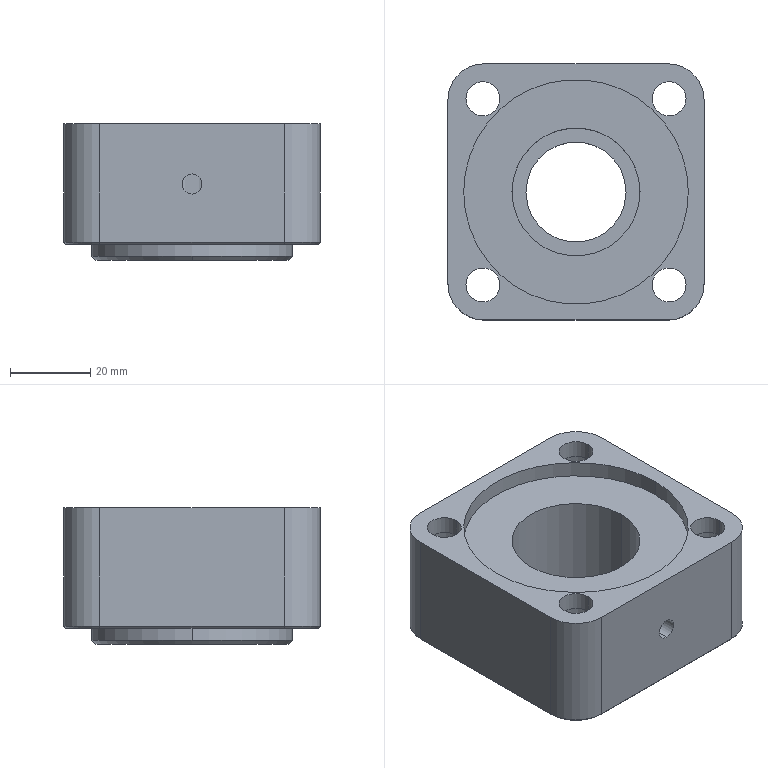Part | SolidWorks | features BaseBody 1 | 1 solid | 53 faces | box 64 x 64 x 34 mm | volume 81907 mm3 | cylinder 30 | plane 17 | cone 6 | commonest cylinder face diameters 8.5 x8 13 x8 18 x4 5 x2 25 x2 32 x2